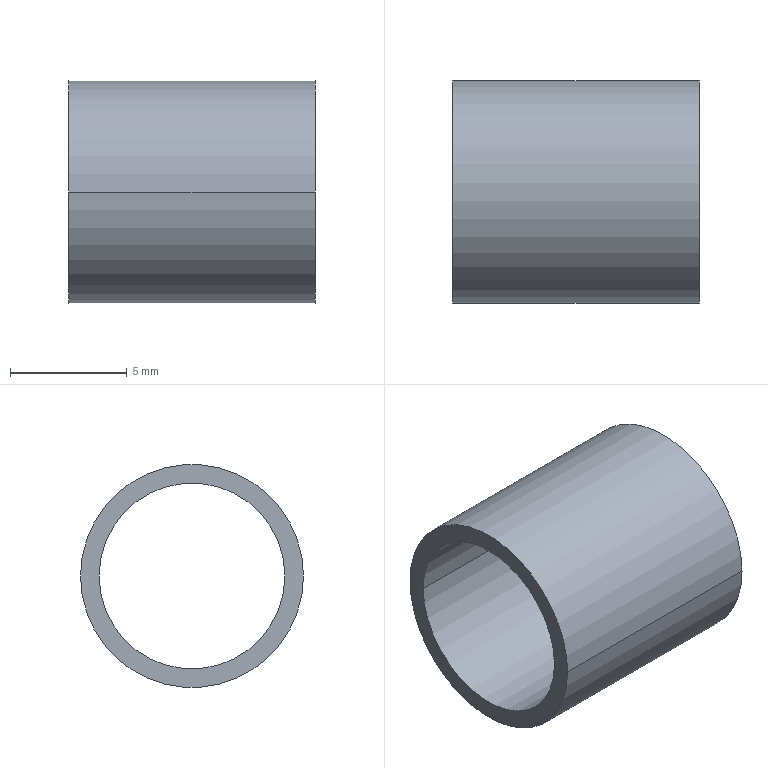Part | NX | features BREP 1 | 1 solid | 6 faces | box 10.541 x 9.525 x 9.525 mm | volume 229.505 mm3 | cylinder 4 | plane 2 | commonest cylinder face diameters 7.938 x2 9.525 x2
STEP:
#1=CARTESIAN_POINT('',(0.,4.763,0.));
#2=VERTEX_POINT('',#1);
#3=CARTESIAN_POINT('',(0.,-4.763,0.));
#4=VERTEX_POINT('',#3);
#5=CARTESIAN_POINT('',(0.,0.,0.));
#6=DIRECTION('',(1.,0.,0.));
#7=DIRECTION('',(0.,1.,0.));
#8=AXIS2_PLACEMENT_3D('',#5,#6,#7);
#9=CIRCLE('',#8,4.763);
#10=EDGE_CURVE('',#2,#4,#9,.T.);
#11=ORIENTED_EDGE('',*,*,#10,.F.);
#12=CARTESIAN_POINT('',(0.,0.,0.));
#13=DIRECTION('',(1.,0.,0.));
#14=DIRECTION('',(0.,-1.,0.));
#15=AXIS2_PLACEMENT_3D('',#12,#13,#14);
#16=CIRCLE('',#15,4.763);
#17=EDGE_CURVE('',#4,#2,#16,.T.);
#18=ORIENTED_EDGE('',*,*,#17,.F.);
#19=EDGE_LOOP('',(#11,#18));
#20=FACE_BOUND('',#19,.T.);
#21=CARTESIAN_POINT('',(0.,-3.969,0.));
#22=VERTEX_POINT('',#21);
#23=CARTESIAN_POINT('',(0.,3.969,0.));
#24=VERTEX_POINT('',#23);
#25=CARTESIAN_POINT('',(0.,0.,0.));
#26=DIRECTION('',(1.,0.,0.));
#27=DIRECTION('',(0.,-1.,0.));
#28=AXIS2_PLACEMENT_3D('',#25,#26,#27);
#29=CIRCLE('',#28,3.969);
#30=EDGE_CURVE('',#22,#24,#29,.T.);
#31=ORIENTED_EDGE('',*,*,#30,.T.);
#32=CARTESIAN_POINT('',(0.,0.,0.));
#33=DIRECTION('',(1.,0.,0.));
#34=DIRECTION('',(0.,1.,0.));
#35=AXIS2_PLACEMENT_3D('',#32,#33,#34);
#36=CIRCLE('',#35,3.969);
#37=EDGE_CURVE('',#24,#22,#36,.T.);
#38=ORIENTED_EDGE('',*,*,#37,.T.);
#39=EDGE_LOOP('',(#31,#38));
#40=FACE_BOUND('',#39,.T.);
#41=CARTESIAN_POINT('',(0.,0.,0.));
#42=DIRECTION('',(1.,0.,0.));
#43=DIRECTION('',(0.,1.,0.));
#44=AXIS2_PLACEMENT_3D('',#41,#42,#43);
#45=PLANE('',#44);
#46=ADVANCED_FACE('',(#20,#40),#45,.F.);
#47=CARTESIAN_POINT('',(10.541,4.763,0.));
#48=VERTEX_POINT('',#47);
#49=CARTESIAN_POINT('',(0.,4.763,0.));
#50=DIRECTION('',(1.,0.,0.));
#51=VECTOR('',#50,1000.);
#52=LINE('',#49,#51);
#53=EDGE_CURVE('',#48,#2,#52,.F.);
#54=ORIENTED_EDGE('',*,*,#53,.F.);
#55=CARTESIAN_POINT('',(10.541,-4.763,0.));
#56=VERTEX_POINT('',#55);
#57=CARTESIAN_POINT('',(10.541,0.,0.));
#58=DIRECTION('',(1.,0.,0.));
#59=DIRECTION('',(0.,-1.,0.));
#60=AXIS2_PLACEMENT_3D('',#57,#58,#59);
#61=CIRCLE('',#60,4.763);
#62=EDGE_CURVE('',#56,#48,#61,.T.);
#63=ORIENTED_EDGE('',*,*,#62,.F.);
#64=CARTESIAN_POINT('',(0.,-4.763,0.));
#65=DIRECTION('',(1.,0.,0.));
#66=VECTOR('',#65,1000.);
#67=LINE('',#64,#66);
#68=EDGE_CURVE('',#56,#4,#67,.F.);
#69=ORIENTED_EDGE('',*,*,#68,.T.);
#70=ORIENTED_EDGE('',*,*,#17,.T.);
#71=EDGE_LOOP('',(#54,#63,#69,#70));
#72=FACE_BOUND('',#71,.T.);
#73=CARTESIAN_POINT('',(0.,0.,0.));
#74=DIRECTION('',(1.,0.,0.));
#75=DIRECTION('',(0.,-1.,0.));
#76=AXIS2_PLACEMENT_3D('',#73,#74,#75);
#77=CYLINDRICAL_SURFACE('',#76,4.763);
#78=ADVANCED_FACE('',(#72),#77,.T.);
#79=ORIENTED_EDGE('',*,*,#68,.F.);
#80=CARTESIAN_POINT('',(10.541,0.,0.));
#81=DIRECTION('',(1.,0.,0.));
#82=DIRECTION('',(0.,1.,0.));
#83=AXIS2_PLACEMENT_3D('',#80,#81,#82);
#84=CIRCLE('',#83,4.763);
#85=EDGE_CURVE('',#48,#56,#84,.T.);
#86=ORIENTED_EDGE('',*,*,#85,.F.);
#87=ORIENTED_EDGE('',*,*,#53,.T.);
#88=ORIENTED_EDGE('',*,*,#10,.T.);
#89=EDGE_LOOP('',(#79,#86,#87,#88));
#90=FACE_BOUND('',#89,.T.);
#91=CARTESIAN_POINT('',(0.,0.,0.));
#92=DIRECTION('',(1.,0.,0.));
#93=DIRECTION('',(0.,-1.,0.));
#94=AXIS2_PLACEMENT_3D('',#91,#92,#93);
#95=CYLINDRICAL_SURFACE('',#94,4.763);
#96=ADVANCED_FACE('',(#90),#95,.T.);
#97=ORIENTED_EDGE('',*,*,#85,.T.);
#98=ORIENTED_EDGE('',*,*,#62,.T.);
#99=EDGE_LOOP('',(#97,#98));
#100=FACE_BOUND('',#99,.T.);
#101=CARTESIAN_POINT('',(10.541,-3.969,0.));
#102=VERTEX_POINT('',#101);
#103=CARTESIAN_POINT('',(10.541,3.969,0.));
#104=VERTEX_POINT('',#103);
#105=CARTESIAN_POINT('',(10.541,0.,0.));
#106=DIRECTION('',(1.,0.,0.));
#107=DIRECTION('',(0.,-1.,0.));
#108=AXIS2_PLACEMENT_3D('',#105,#106,#107);
#109=CIRCLE('',#108,3.969);
#110=EDGE_CURVE('',#102,#104,#109,.T.);
#111=ORIENTED_EDGE('',*,*,#110,.F.);
#112=CARTESIAN_POINT('',(10.541,0.,0.));
#113=DIRECTION('',(1.,0.,0.));
#114=DIRECTION('',(0.,1.,0.));
#115=AXIS2_PLACEMENT_3D('',#112,#113,#114);
#116=CIRCLE('',#115,3.969);
#117=EDGE_CURVE('',#104,#102,#116,.T.);
#118=ORIENTED_EDGE('',*,*,#117,.F.);
#119=EDGE_LOOP('',(#111,#118));
#120=FACE_BOUND('',#119,.T.);
#121=CARTESIAN_POINT('',(10.541,0.,0.));
#122=DIRECTION('',(1.,0.,0.));
#123=DIRECTION('',(0.,1.,0.));
#124=AXIS2_PLACEMENT_3D('',#121,#122,#123);
#125=PLANE('',#124);
#126=ADVANCED_FACE('',(#100,#120),#125,.T.);
#127=CARTESIAN_POINT('',(0.,3.969,0.));
#128=DIRECTION('',(1.,0.,0.));
#129=VECTOR('',#128,1000.);
#130=LINE('',#127,#129);
#131=EDGE_CURVE('',#104,#24,#130,.F.);
#132=ORIENTED_EDGE('',*,*,#131,.F.);
#133=ORIENTED_EDGE('',*,*,#117,.T.);
#134=CARTESIAN_POINT('',(0.,-3.969,0.));
#135=DIRECTION('',(1.,0.,0.));
#136=VECTOR('',#135,1000.);
#137=LINE('',#134,#136);
#138=EDGE_CURVE('',#102,#22,#137,.F.);
#139=ORIENTED_EDGE('',*,*,#138,.T.);
#140=ORIENTED_EDGE('',*,*,#37,.F.);
#141=EDGE_LOOP('',(#132,#133,#139,#140));
#142=FACE_BOUND('',#141,.T.);
#143=CARTESIAN_POINT('',(0.,0.,0.));
#144=DIRECTION('',(1.,0.,0.));
#145=DIRECTION('',(0.,1.,0.));
#146=AXIS2_PLACEMENT_3D('',#143,#144,#145);
#147=CYLINDRICAL_SURFACE('',#146,3.969);
#148=ADVANCED_FACE('',(#142),#147,.F.);
#149=ORIENTED_EDGE('',*,*,#138,.F.);
#150=ORIENTED_EDGE('',*,*,#110,.T.);
#151=ORIENTED_EDGE('',*,*,#131,.T.);
#152=ORIENTED_EDGE('',*,*,#30,.F.);
#153=EDGE_LOOP('',(#149,#150,#151,#152));
#154=FACE_BOUND('',#153,.T.);
#155=CARTESIAN_POINT('',(0.,0.,0.));
#156=DIRECTION('',(1.,0.,0.));
#157=DIRECTION('',(0.,1.,0.));
#158=AXIS2_PLACEMENT_3D('',#155,#156,#157);
#159=CYLINDRICAL_SURFACE('',#158,3.969);
#160=ADVANCED_FACE('',(#154),#159,.F.);
#161=CLOSED_SHELL('',(#46,#78,#96,#126,#148,#160));
#162=MANIFOLD_SOLID_BREP('',#161);
#163=(LENGTH_UNIT()NAMED_UNIT(*)SI_UNIT(.MILLI.,.METRE.));
#164=UNCERTAINTY_MEASURE_WITH_UNIT(LENGTH_MEASURE(0.00001),#163,'','');
#165=(NAMED_UNIT(*)PLANE_ANGLE_UNIT()SI_UNIT($,.RADIAN.));
#166=(NAMED_UNIT(*)SI_UNIT($,.STERADIAN.)SOLID_ANGLE_UNIT());
#167=(GEOMETRIC_REPRESENTATION_CONTEXT(3)GLOBAL_UNCERTAINTY_ASSIGNED_CONTEXT((#164))GLOBAL_UNIT_ASSIGNED_CONTEXT((#163,#165,#166))REPRESENTATION_CONTEXT('',''));
#168=ADVANCED_BREP_SHAPE_REPRESENTATION('',(#162),#167);